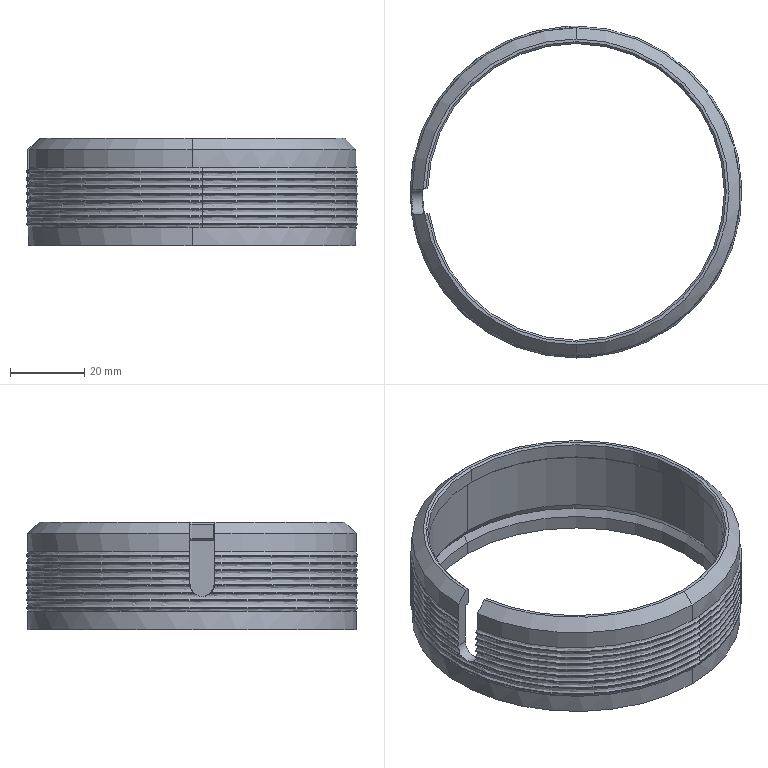Part | SolidWorks | features BaseBody 1 | 1 solid | 77 faces | box 89.5 x 89.5 x 29 mm | volume 22014 mm3 | cylinder 35 | spline 24 | cone 13 | plane 5 | commonest cylinder face diameters 89.5 x22 88.5 x5 83 x4 80 x3 6.7 x1